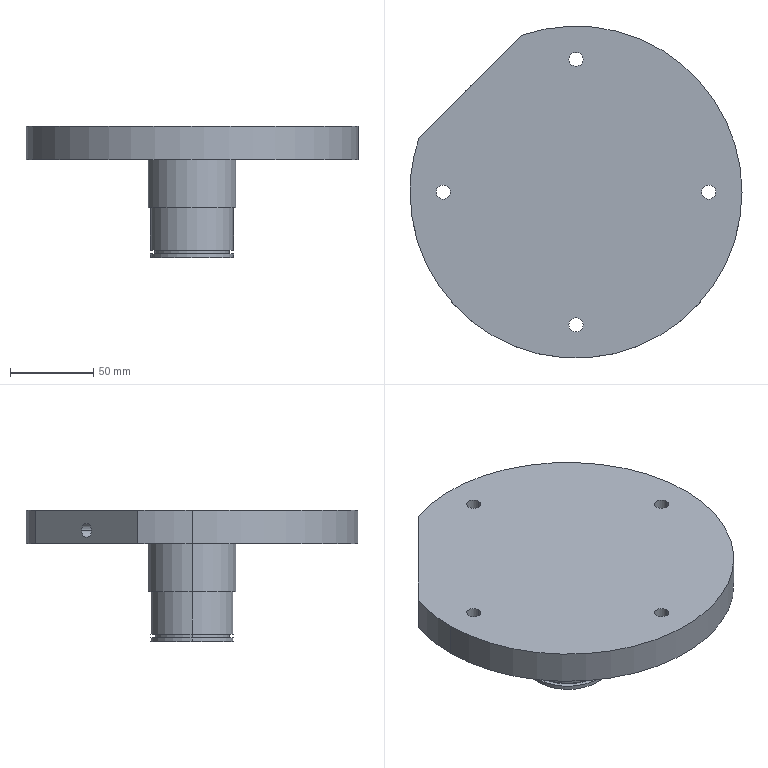Part | SolidWorks | features HoleWzd 2, ICE 2, CirPattern 1, Revolution 1 | 1 solid | 30 faces | box 200 x 200 x 79.02 mm | volume 730688 mm3 | cylinder 21 | plane 7 | cone 2 | commonest cylinder face diameters 8.5 x10 50 x4 200 x3 45 x2 53 x2
STEP:
#1=CARTESIAN_POINT('',(-18.208,24.218,-12.));
#2=VERTEX_POINT('',#1);
#3=CARTESIAN_POINT('',(-24.218,18.208,-12.));
#4=VERTEX_POINT('',#3);
#5=CARTESIAN_POINT('',(-21.213,21.213,-12.));
#6=DIRECTION('',(-0.7071,0.7071,0.));
#7=DIRECTION('',(-0.7071,-0.7071,0.));
#8=AXIS2_PLACEMENT_3D('',#5,#6,#7);
#9=CIRCLE('',#8,4.25);
#10=EDGE_CURVE('',#2,#4,#9,.T.);
#11=ORIENTED_EDGE('',*,*,#10,.F.);
#12=CARTESIAN_POINT('',(-60.634,66.645,-12.));
#13=VERTEX_POINT('',#12);
#14=CARTESIAN_POINT('',(-60.634,66.645,-12.));
#15=DIRECTION('',(-0.7071,0.7071,0.));
#16=VECTOR('',#15,1000.);
#17=LINE('',#14,#16);
#18=EDGE_CURVE('',#2,#13,#17,.T.);
#19=ORIENTED_EDGE('',*,*,#18,.T.);
#20=CARTESIAN_POINT('',(-66.645,60.634,-12.));
#21=VERTEX_POINT('',#20);
#22=CARTESIAN_POINT('',(-63.64,63.64,-12.));
#23=DIRECTION('',(-0.7071,0.7071,0.));
#24=DIRECTION('',(-0.7071,-0.7071,0.));
#25=AXIS2_PLACEMENT_3D('',#22,#23,#24);
#26=CIRCLE('',#25,4.25);
#27=EDGE_CURVE('',#13,#21,#26,.T.);
#28=ORIENTED_EDGE('',*,*,#27,.T.);
#29=CARTESIAN_POINT('',(-66.645,60.634,-12.));
#30=DIRECTION('',(-0.7071,0.7071,0.));
#31=VECTOR('',#30,1000.);
#32=LINE('',#29,#31);
#33=EDGE_CURVE('',#4,#21,#32,.T.);
#34=ORIENTED_EDGE('',*,*,#33,.F.);
#35=EDGE_LOOP('',(#11,#19,#28,#34));
#36=FACE_OUTER_BOUND('',#35,.T.);
#37=CARTESIAN_POINT('',(-63.64,63.64,-12.));
#38=DIRECTION('',(-0.7071,0.7071,0.));
#39=DIRECTION('',(-0.7071,-0.7071,0.));
#40=AXIS2_PLACEMENT_3D('',#37,#38,#39);
#41=CYLINDRICAL_SURFACE('',#40,4.25);
#42=ADVANCED_FACE('',(#36),#41,.F.);
#43=CARTESIAN_POINT('',(-19.407,19.407,-12.));
#44=VERTEX_POINT('',#43);
#45=CARTESIAN_POINT('',(-24.218,18.208,-12.));
#46=DIRECTION('',(-0.9703,-0.2419,0.));
#47=VECTOR('',#46,1000.);
#48=LINE('',#45,#47);
#49=EDGE_CURVE('',#44,#4,#48,.T.);
#50=ORIENTED_EDGE('',*,*,#49,.F.);
#51=CARTESIAN_POINT('',(-18.208,24.218,-12.));
#52=DIRECTION('',(0.2419,0.9703,0.));
#53=VECTOR('',#52,1000.);
#54=LINE('',#51,#53);
#55=EDGE_CURVE('',#44,#2,#54,.T.);
#56=ORIENTED_EDGE('',*,*,#55,.T.);
#57=ORIENTED_EDGE('',*,*,#10,.T.);
#58=EDGE_LOOP('',(#50,#56,#57));
#59=FACE_OUTER_BOUND('',#58,.T.);
#60=CARTESIAN_POINT('',(-21.213,21.213,-12.));
#61=DIRECTION('',(-0.7071,0.7071,0.));
#62=DIRECTION('',(-0.7071,-0.7071,0.));
#63=AXIS2_PLACEMENT_3D('',#60,#61,#62);
#64=CONICAL_SURFACE('',#63,4.25,1.03);
#65=ADVANCED_FACE('',(#59),#64,.F.);
#66=CARTESIAN_POINT('',(84.25,0.,0.));
#67=VERTEX_POINT('',#66);
#68=CARTESIAN_POINT('',(75.75,0.,0.));
#69=VERTEX_POINT('',#68);
#70=CARTESIAN_POINT('',(80.,0.,0.));
#71=DIRECTION('',(0.,0.,-1.));
#72=DIRECTION('',(-1.,0.,0.));
#73=AXIS2_PLACEMENT_3D('',#70,#71,#72);
#74=CIRCLE('',#73,4.25);
#75=EDGE_CURVE('',#67,#69,#74,.T.);
#76=ORIENTED_EDGE('',*,*,#75,.F.);
#77=CARTESIAN_POINT('',(84.25,0.,-20.));
#78=VERTEX_POINT('',#77);
#79=CARTESIAN_POINT('',(84.25,0.,-20.));
#80=DIRECTION('',(0.,0.,-1.));
#81=VECTOR('',#80,1000.);
#82=LINE('',#79,#81);
#83=EDGE_CURVE('',#67,#78,#82,.T.);
#84=ORIENTED_EDGE('',*,*,#83,.T.);
#85=CARTESIAN_POINT('',(75.75,0.,-20.));
#86=VERTEX_POINT('',#85);
#87=CARTESIAN_POINT('',(80.,0.,-20.));
#88=DIRECTION('',(0.,0.,-1.));
#89=DIRECTION('',(-1.,0.,0.));
#90=AXIS2_PLACEMENT_3D('',#87,#88,#89);
#91=CIRCLE('',#90,4.25);
#92=EDGE_CURVE('',#78,#86,#91,.T.);
#93=ORIENTED_EDGE('',*,*,#92,.T.);
#94=CARTESIAN_POINT('',(75.75,0.,-20.));
#95=DIRECTION('',(0.,0.,-1.));
#96=VECTOR('',#95,1000.);
#97=LINE('',#94,#96);
#98=EDGE_CURVE('',#69,#86,#97,.T.);
#99=ORIENTED_EDGE('',*,*,#98,.F.);
#100=EDGE_LOOP('',(#76,#84,#93,#99));
#101=FACE_OUTER_BOUND('',#100,.T.);
#102=CARTESIAN_POINT('',(80.,0.,-20.));
#103=DIRECTION('',(0.,0.,-1.));
#104=DIRECTION('',(-1.,0.,0.));
#105=AXIS2_PLACEMENT_3D('',#102,#103,#104);
#106=CYLINDRICAL_SURFACE('',#105,4.25);
#107=ADVANCED_FACE('',(#101),#106,.F.);
#108=CARTESIAN_POINT('',(4.25,80.,0.));
#109=VERTEX_POINT('',#108);
#110=CARTESIAN_POINT('',(-4.25,80.,0.));
#111=VERTEX_POINT('',#110);
#112=CARTESIAN_POINT('',(0.,80.,0.));
#113=DIRECTION('',(0.,0.,-1.));
#114=DIRECTION('',(-1.,0.,0.));
#115=AXIS2_PLACEMENT_3D('',#112,#113,#114);
#116=CIRCLE('',#115,4.25);
#117=EDGE_CURVE('',#109,#111,#116,.T.);
#118=ORIENTED_EDGE('',*,*,#117,.F.);
#119=CARTESIAN_POINT('',(4.25,80.,-20.));
#120=VERTEX_POINT('',#119);
#121=CARTESIAN_POINT('',(4.25,80.,-20.));
#122=DIRECTION('',(0.,0.,-1.));
#123=VECTOR('',#122,1000.);
#124=LINE('',#121,#123);
#125=EDGE_CURVE('',#109,#120,#124,.T.);
#126=ORIENTED_EDGE('',*,*,#125,.T.);
#127=CARTESIAN_POINT('',(-4.25,80.,-20.));
#128=VERTEX_POINT('',#127);
#129=CARTESIAN_POINT('',(0.,80.,-20.));
#130=DIRECTION('',(0.,0.,-1.));
#131=DIRECTION('',(-1.,0.,0.));
#132=AXIS2_PLACEMENT_3D('',#129,#130,#131);
#133=CIRCLE('',#132,4.25);
#134=EDGE_CURVE('',#120,#128,#133,.T.);
#135=ORIENTED_EDGE('',*,*,#134,.T.);
#136=CARTESIAN_POINT('',(-4.25,80.,-20.));
#137=DIRECTION('',(0.,0.,-1.));
#138=VECTOR('',#137,1000.);
#139=LINE('',#136,#138);
#140=EDGE_CURVE('',#111,#128,#139,.T.);
#141=ORIENTED_EDGE('',*,*,#140,.F.);
#142=EDGE_LOOP('',(#118,#126,#135,#141));
#143=FACE_OUTER_BOUND('',#142,.T.);
#144=CARTESIAN_POINT('',(0.,80.,-20.));
#145=DIRECTION('',(0.,0.,-1.));
#146=DIRECTION('',(-1.,0.,0.));
#147=AXIS2_PLACEMENT_3D('',#144,#145,#146);
#148=CYLINDRICAL_SURFACE('',#147,4.25);
#149=ADVANCED_FACE('',(#143),#148,.F.);
#150=CARTESIAN_POINT('',(-75.75,0.,0.));
#151=VERTEX_POINT('',#150);
#152=CARTESIAN_POINT('',(-84.25,0.,0.));
#153=VERTEX_POINT('',#152);
#154=CARTESIAN_POINT('',(-80.,0.,0.));
#155=DIRECTION('',(0.,0.,-1.));
#156=DIRECTION('',(-1.,0.,0.));
#157=AXIS2_PLACEMENT_3D('',#154,#155,#156);
#158=CIRCLE('',#157,4.25);
#159=EDGE_CURVE('',#151,#153,#158,.T.);
#160=ORIENTED_EDGE('',*,*,#159,.F.);
#161=CARTESIAN_POINT('',(-75.75,0.,-20.));
#162=VERTEX_POINT('',#161);
#163=CARTESIAN_POINT('',(-75.75,0.,-20.));
#164=DIRECTION('',(0.,0.,-1.));
#165=VECTOR('',#164,1000.);
#166=LINE('',#163,#165);
#167=EDGE_CURVE('',#151,#162,#166,.T.);
#168=ORIENTED_EDGE('',*,*,#167,.T.);
#169=CARTESIAN_POINT('',(-84.25,0.,-20.));
#170=VERTEX_POINT('',#169);
#171=CARTESIAN_POINT('',(-80.,0.,-20.));
#172=DIRECTION('',(0.,0.,-1.));
#173=DIRECTION('',(-1.,0.,0.));
#174=AXIS2_PLACEMENT_3D('',#171,#172,#173);
#175=CIRCLE('',#174,4.25);
#176=EDGE_CURVE('',#162,#170,#175,.T.);
#177=ORIENTED_EDGE('',*,*,#176,.T.);
#178=CARTESIAN_POINT('',(-84.25,0.,-20.));
#179=DIRECTION('',(0.,0.,-1.));
#180=VECTOR('',#179,1000.);
#181=LINE('',#178,#180);
#182=EDGE_CURVE('',#153,#170,#181,.T.);
#183=ORIENTED_EDGE('',*,*,#182,.F.);
#184=EDGE_LOOP('',(#160,#168,#177,#183));
#185=FACE_OUTER_BOUND('',#184,.T.);
#186=CARTESIAN_POINT('',(-80.,0.,-20.));
#187=DIRECTION('',(0.,0.,-1.));
#188=DIRECTION('',(-1.,0.,0.));
#189=AXIS2_PLACEMENT_3D('',#186,#187,#188);
#190=CYLINDRICAL_SURFACE('',#189,4.25);
#191=ADVANCED_FACE('',(#185),#190,.F.);
#192=CARTESIAN_POINT('',(4.25,-80.,0.));
#193=VERTEX_POINT('',#192);
#194=CARTESIAN_POINT('',(-4.25,-80.,0.));
#195=VERTEX_POINT('',#194);
#196=CARTESIAN_POINT('',(0.,-80.,0.));
#197=DIRECTION('',(0.,0.,-1.));
#198=DIRECTION('',(-1.,0.,0.));
#199=AXIS2_PLACEMENT_3D('',#196,#197,#198);
#200=CIRCLE('',#199,4.25);
#201=EDGE_CURVE('',#193,#195,#200,.T.);
#202=ORIENTED_EDGE('',*,*,#201,.F.);
#203=CARTESIAN_POINT('',(4.25,-80.,-20.));
#204=VERTEX_POINT('',#203);
#205=CARTESIAN_POINT('',(4.25,-80.,-20.));
#206=DIRECTION('',(0.,0.,-1.));
#207=VECTOR('',#206,1000.);
#208=LINE('',#205,#207);
#209=EDGE_CURVE('',#193,#204,#208,.T.);
#210=ORIENTED_EDGE('',*,*,#209,.T.);
#211=CARTESIAN_POINT('',(-4.25,-80.,-20.));
#212=VERTEX_POINT('',#211);
#213=CARTESIAN_POINT('',(0.,-80.,-20.));
#214=DIRECTION('',(0.,0.,-1.));
#215=DIRECTION('',(-1.,0.,0.));
#216=AXIS2_PLACEMENT_3D('',#213,#214,#215);
#217=CIRCLE('',#216,4.25);
#218=EDGE_CURVE('',#204,#212,#217,.T.);
#219=ORIENTED_EDGE('',*,*,#218,.T.);
#220=CARTESIAN_POINT('',(-4.25,-80.,-20.));
#221=DIRECTION('',(0.,0.,-1.));
#222=VECTOR('',#221,1000.);
#223=LINE('',#220,#222);
#224=EDGE_CURVE('',#195,#212,#223,.T.);
#225=ORIENTED_EDGE('',*,*,#224,.F.);
#226=EDGE_LOOP('',(#202,#210,#219,#225));
#227=FACE_OUTER_BOUND('',#226,.T.);
#228=CARTESIAN_POINT('',(0.,-80.,-20.));
#229=DIRECTION('',(0.,0.,-1.));
#230=DIRECTION('',(-1.,0.,0.));
#231=AXIS2_PLACEMENT_3D('',#228,#229,#230);
#232=CYLINDRICAL_SURFACE('',#231,4.25);
#233=ADVANCED_FACE('',(#227),#232,.F.);
#234=CARTESIAN_POINT('',(25.,0.,-76.72));
#235=VERTEX_POINT('',#234);
#236=CARTESIAN_POINT('',(-25.,0.,-76.72));
#237=VERTEX_POINT('',#236);
#238=CARTESIAN_POINT('',(0.,0.,-76.72));
#239=DIRECTION('',(0.,0.,1.));
#240=DIRECTION('',(-1.,0.,0.));
#241=AXIS2_PLACEMENT_3D('',#238,#239,#240);
#242=CIRCLE('',#241,25.);
#243=EDGE_CURVE('',#235,#237,#242,.T.);
#244=ORIENTED_EDGE('',*,*,#243,.F.);
#245=CARTESIAN_POINT('',(25.,0.,-79.02));
#246=VERTEX_POINT('',#245);
#247=CARTESIAN_POINT('',(25.,0.,0.));
#248=DIRECTION('',(0.,0.,-1.));
#249=VECTOR('',#248,1000.);
#250=LINE('',#247,#249);
#251=EDGE_CURVE('',#235,#246,#250,.T.);
#252=ORIENTED_EDGE('',*,*,#251,.T.);
#253=CARTESIAN_POINT('',(-25.,0.,-79.02));
#254=VERTEX_POINT('',#253);
#255=CARTESIAN_POINT('',(0.,0.,-79.02));
#256=DIRECTION('',(0.,0.,-1.));
#257=DIRECTION('',(-1.,0.,0.));
#258=AXIS2_PLACEMENT_3D('',#255,#256,#257);
#259=CIRCLE('',#258,25.);
#260=EDGE_CURVE('',#254,#246,#259,.T.);
#261=ORIENTED_EDGE('',*,*,#260,.F.);
#262=CARTESIAN_POINT('',(-25.,0.,0.));
#263=DIRECTION('',(0.,0.,-1.));
#264=VECTOR('',#263,1000.);
#265=LINE('',#262,#264);
#266=EDGE_CURVE('',#237,#254,#265,.T.);
#267=ORIENTED_EDGE('',*,*,#266,.F.);
#268=EDGE_LOOP('',(#244,#252,#261,#267));
#269=FACE_OUTER_BOUND('',#268,.T.);
#270=CARTESIAN_POINT('',(0.,0.,0.));
#271=DIRECTION('',(0.,0.,-1.));
#272=DIRECTION('',(-1.,0.,0.));
#273=AXIS2_PLACEMENT_3D('',#270,#271,#272);
#274=CYLINDRICAL_SURFACE('',#273,25.);
#275=ADVANCED_FACE('',(#269),#274,.T.);
#276=CARTESIAN_POINT('',(-22.5,0.,-76.72));
#277=VERTEX_POINT('',#276);
#278=CARTESIAN_POINT('',(22.5,0.,-76.72));
#279=VERTEX_POINT('',#278);
#280=CARTESIAN_POINT('',(0.,0.,-76.72));
#281=DIRECTION('',(0.,0.,-1.));
#282=DIRECTION('',(-1.,0.,0.));
#283=AXIS2_PLACEMENT_3D('',#280,#281,#282);
#284=CIRCLE('',#283,22.5);
#285=EDGE_CURVE('',#277,#279,#284,.T.);
#286=ORIENTED_EDGE('',*,*,#285,.F.);
#287=CARTESIAN_POINT('',(-22.5,0.,-74.52));
#288=VERTEX_POINT('',#287);
#289=CARTESIAN_POINT('',(-22.5,0.,-76.72));
#290=DIRECTION('',(0.,0.,1.));
#291=VECTOR('',#290,1000.);
#292=LINE('',#289,#291);
#293=EDGE_CURVE('',#277,#288,#292,.T.);
#294=ORIENTED_EDGE('',*,*,#293,.T.);
#295=CARTESIAN_POINT('',(22.5,0.,-74.52));
#296=VERTEX_POINT('',#295);
#297=CARTESIAN_POINT('',(0.,0.,-74.52));
#298=DIRECTION('',(0.,0.,-1.));
#299=DIRECTION('',(-1.,0.,0.));
#300=AXIS2_PLACEMENT_3D('',#297,#298,#299);
#301=CIRCLE('',#300,22.5);
#302=EDGE_CURVE('',#288,#296,#301,.T.);
#303=ORIENTED_EDGE('',*,*,#302,.T.);
#304=CARTESIAN_POINT('',(22.5,0.,-76.72));
#305=DIRECTION('',(0.,0.,1.));
#306=VECTOR('',#305,1000.);
#307=LINE('',#304,#306);
#308=EDGE_CURVE('',#279,#296,#307,.T.);
#309=ORIENTED_EDGE('',*,*,#308,.F.);
#310=EDGE_LOOP('',(#286,#294,#303,#309));
#311=FACE_OUTER_BOUND('',#310,.T.);
#312=CARTESIAN_POINT('',(0.,0.,-76.72));
#313=DIRECTION('',(0.,0.,1.));
#314=DIRECTION('',(1.,0.,0.));
#315=AXIS2_PLACEMENT_3D('',#312,#313,#314);
#316=CYLINDRICAL_SURFACE('',#315,22.5);
#317=ADVANCED_FACE('',(#311),#316,.T.);
#318=CARTESIAN_POINT('',(-26.5,0.,-20.));
#319=VERTEX_POINT('',#318);
#320=CARTESIAN_POINT('',(26.5,0.,-20.));
#321=VERTEX_POINT('',#320);
#322=CARTESIAN_POINT('',(0.,0.,-20.));
#323=DIRECTION('',(0.,0.,-1.));
#324=DIRECTION('',(-1.,0.,0.));
#325=AXIS2_PLACEMENT_3D('',#322,#323,#324);
#326=CIRCLE('',#325,26.5);
#327=EDGE_CURVE('',#319,#321,#326,.T.);
#328=ORIENTED_EDGE('',*,*,#327,.T.);
#329=CARTESIAN_POINT('',(26.5,0.,-49.02));
#330=VERTEX_POINT('',#329);
#331=CARTESIAN_POINT('',(26.5,0.,0.));
#332=DIRECTION('',(0.,0.,-1.));
#333=VECTOR('',#332,1000.);
#334=LINE('',#331,#333);
#335=EDGE_CURVE('',#321,#330,#334,.T.);
#336=ORIENTED_EDGE('',*,*,#335,.T.);
#337=CARTESIAN_POINT('',(-26.5,0.,-49.02));
#338=VERTEX_POINT('',#337);
#339=CARTESIAN_POINT('',(0.,0.,-49.02));
#340=DIRECTION('',(0.,0.,-1.));
#341=DIRECTION('',(-1.,0.,0.));
#342=AXIS2_PLACEMENT_3D('',#339,#340,#341);
#343=CIRCLE('',#342,26.5);
#344=EDGE_CURVE('',#338,#330,#343,.T.);
#345=ORIENTED_EDGE('',*,*,#344,.F.);
#346=CARTESIAN_POINT('',(-26.5,0.,0.));
#347=DIRECTION('',(0.,0.,-1.));
#348=VECTOR('',#347,1000.);
#349=LINE('',#346,#348);
#350=EDGE_CURVE('',#319,#338,#349,.T.);
#351=ORIENTED_EDGE('',*,*,#350,.F.);
#352=EDGE_LOOP('',(#328,#336,#345,#351));
#353=FACE_OUTER_BOUND('',#352,.T.);
#354=CARTESIAN_POINT('',(0.,0.,0.));
#355=DIRECTION('',(0.,0.,-1.));
#356=DIRECTION('',(-1.,0.,0.));
#357=AXIS2_PLACEMENT_3D('',#354,#355,#356);
#358=CYLINDRICAL_SURFACE('',#357,26.5);
#359=ADVANCED_FACE('',(#353),#358,.T.);
#360=CARTESIAN_POINT('',(-32.818,94.462,0.));
#361=VERTEX_POINT('',#360);
#362=CARTESIAN_POINT('',(100.,0.,0.));
#363=VERTEX_POINT('',#362);
#364=CARTESIAN_POINT('',(0.,0.,0.));
#365=DIRECTION('',(0.,0.,-1.));
#366=DIRECTION('',(-1.,0.,0.));
#367=AXIS2_PLACEMENT_3D('',#364,#365,#366);
#368=CIRCLE('',#367,100.);
#369=EDGE_CURVE('',#361,#363,#368,.T.);
#370=ORIENTED_EDGE('',*,*,#369,.T.);
#371=CARTESIAN_POINT('',(100.,0.,-20.));
#372=VERTEX_POINT('',#371);
#373=CARTESIAN_POINT('',(100.,0.,0.));
#374=DIRECTION('',(0.,0.,-1.));
#375=VECTOR('',#374,1000.);
#376=LINE('',#373,#375);
#377=EDGE_CURVE('',#363,#372,#376,.T.);
#378=ORIENTED_EDGE('',*,*,#377,.T.);
#379=CARTESIAN_POINT('',(-32.818,94.462,-20.));
#380=VERTEX_POINT('',#379);
#381=CARTESIAN_POINT('',(0.,0.,-20.));
#382=DIRECTION('',(0.,0.,-1.));
#383=DIRECTION('',(-1.,0.,0.));
#384=AXIS2_PLACEMENT_3D('',#381,#382,#383);
#385=CIRCLE('',#384,100.);
#386=EDGE_CURVE('',#380,#372,#385,.T.);
#387=ORIENTED_EDGE('',*,*,#386,.F.);
#388=CARTESIAN_POINT('',(-32.818,94.462,0.));
#389=DIRECTION('',(0.,0.,-1.));
#390=VECTOR('',#389,1000.);
#391=LINE('',#388,#390);
#392=EDGE_CURVE('',#361,#380,#391,.T.);
#393=ORIENTED_EDGE('',*,*,#392,.F.);
#394=EDGE_LOOP('',(#370,#378,#387,#393));
#395=FACE_OUTER_BOUND('',#394,.T.);
#396=CARTESIAN_POINT('',(0.,0.,0.));
#397=DIRECTION('',(0.,0.,-1.));
#398=DIRECTION('',(-1.,0.,0.));
#399=AXIS2_PLACEMENT_3D('',#396,#397,#398);
#400=CYLINDRICAL_SURFACE('',#399,100.);
#401=ADVANCED_FACE('',(#395),#400,.T.);
#402=ORIENTED_EDGE('',*,*,#377,.F.);
#403=CARTESIAN_POINT('',(-100.,0.,0.));
#404=VERTEX_POINT('',#403);
#405=CARTESIAN_POINT('',(0.,0.,0.));
#406=DIRECTION('',(0.,0.,-1.));
#407=DIRECTION('',(-1.,0.,0.));
#408=AXIS2_PLACEMENT_3D('',#405,#406,#407);
#409=CIRCLE('',#408,100.);
#410=EDGE_CURVE('',#363,#404,#409,.T.);
#411=ORIENTED_EDGE('',*,*,#410,.T.);
#412=CARTESIAN_POINT('',(-100.,0.,-20.));
#413=VERTEX_POINT('',#412);
#414=CARTESIAN_POINT('',(-100.,0.,0.));
#415=DIRECTION('',(0.,0.,-1.));
#416=VECTOR('',#415,1000.);
#417=LINE('',#414,#416);
#418=EDGE_CURVE('',#404,#413,#417,.T.);
#419=ORIENTED_EDGE('',*,*,#418,.T.);
#420=CARTESIAN_POINT('',(0.,0.,-20.));
#421=DIRECTION('',(0.,0.,-1.));
#422=DIRECTION('',(-1.,0.,0.));
#423=AXIS2_PLACEMENT_3D('',#420,#421,#422);
#424=CIRCLE('',#423,100.);
#425=EDGE_CURVE('',#372,#413,#424,.T.);
#426=ORIENTED_EDGE('',*,*,#425,.F.);
#427=EDGE_LOOP('',(#402,#411,#419,#426));
#428=FACE_OUTER_BOUND('',#427,.T.);
#429=CARTESIAN_POINT('',(0.,0.,0.));
#430=DIRECTION('',(0.,0.,-1.));
#431=DIRECTION('',(-1.,0.,0.));
#432=AXIS2_PLACEMENT_3D('',#429,#430,#431);
#433=CYLINDRICAL_SURFACE('',#432,100.);
#434=ADVANCED_FACE('',(#428),#433,.T.);
#435=CARTESIAN_POINT('',(-25.,0.,-49.02));
#436=VERTEX_POINT('',#435);
#437=CARTESIAN_POINT('',(25.,0.,-49.02));
#438=VERTEX_POINT('',#437);
#439=CARTESIAN_POINT('',(0.,0.,-49.02));
#440=DIRECTION('',(0.,0.,-1.));
#441=DIRECTION('',(-1.,0.,0.));
#442=AXIS2_PLACEMENT_3D('',#439,#440,#441);
#443=CIRCLE('',#442,25.);
#444=EDGE_CURVE('',#436,#438,#443,.T.);
#445=ORIENTED_EDGE('',*,*,#444,.T.);
#446=CARTESIAN_POINT('',(25.,0.,-74.52));
#447=VERTEX_POINT('',#446);
#448=CARTESIAN_POINT('',(25.,0.,0.));
#449=DIRECTION('',(0.,0.,-1.));
#450=VECTOR('',#449,1000.);
#451=LINE('',#448,#450);
#452=EDGE_CURVE('',#438,#447,#451,.T.);
#453=ORIENTED_EDGE('',*,*,#452,.T.);
#454=CARTESIAN_POINT('',(-25.,0.,-74.52));
#455=VERTEX_POINT('',#454);
#456=CARTESIAN_POINT('',(0.,0.,-74.52));
#457=DIRECTION('',(0.,0.,1.));
#458=DIRECTION('',(-1.,0.,0.));
#459=AXIS2_PLACEMENT_3D('',#456,#457,#458);
#460=CIRCLE('',#459,25.);
#461=EDGE_CURVE('',#447,#455,#460,.T.);
#462=ORIENTED_EDGE('',*,*,#461,.T.);
#463=CARTESIAN_POINT('',(-25.,0.,0.));
#464=DIRECTION('',(0.,0.,-1.));
#465=VECTOR('',#464,1000.);
#466=LINE('',#463,#465);
#467=EDGE_CURVE('',#436,#455,#466,.T.);
#468=ORIENTED_EDGE('',*,*,#467,.F.);
#469=EDGE_LOOP('',(#445,#453,#462,#468));
#470=FACE_OUTER_BOUND('',#469,.T.);
#471=CARTESIAN_POINT('',(0.,0.,0.));
#472=DIRECTION('',(0.,0.,-1.));
#473=DIRECTION('',(-1.,0.,0.));
#474=AXIS2_PLACEMENT_3D('',#471,#472,#473);
#475=CYLINDRICAL_SURFACE('',#474,25.);
#476=ADVANCED_FACE('',(#470),#475,.T.);
#477=ORIENTED_EDGE('',*,*,#452,.F.);
#478=CARTESIAN_POINT('',(0.,0.,-49.02));
#479=DIRECTION('',(0.,0.,-1.));
#480=DIRECTION('',(-1.,0.,0.));
#481=AXIS2_PLACEMENT_3D('',#478,#479,#480);
#482=CIRCLE('',#481,25.);
#483=EDGE_CURVE('',#438,#436,#482,.T.);
#484=ORIENTED_EDGE('',*,*,#483,.T.);
#485=ORIENTED_EDGE('',*,*,#467,.T.);
#486=CARTESIAN_POINT('',(0.,0.,-74.52));
#487=DIRECTION('',(0.,0.,1.));
#488=DIRECTION('',(-1.,0.,0.));
#489=AXIS2_PLACEMENT_3D('',#486,#487,#488);
#490=CIRCLE('',#489,25.);
#491=EDGE_CURVE('',#455,#447,#490,.T.);
#492=ORIENTED_EDGE('',*,*,#491,.T.);
#493=EDGE_LOOP('',(#477,#484,#485,#492));
#494=FACE_OUTER_BOUND('',#493,.T.);
#495=CARTESIAN_POINT('',(0.,0.,0.));
#496=DIRECTION('',(0.,0.,-1.));
#497=DIRECTION('',(-1.,0.,0.));
#498=AXIS2_PLACEMENT_3D('',#495,#496,#497);
#499=CYLINDRICAL_SURFACE('',#498,25.);
#500=ADVANCED_FACE('',(#494),#499,.T.);
#501=CARTESIAN_POINT('',(-94.462,32.818,0.));
#502=VERTEX_POINT('',#501);
#503=CARTESIAN_POINT('',(-106.066,21.213,0.));
#504=DIRECTION('',(-0.7071,-0.7071,0.));
#505=VECTOR('',#504,1000.);
#506=LINE('',#503,#505);
#507=EDGE_CURVE('',#361,#502,#506,.T.);
#508=ORIENTED_EDGE('',*,*,#507,.T.);
#509=CARTESIAN_POINT('',(0.,0.,0.));
#510=DIRECTION('',(0.,0.,-1.));
#511=DIRECTION('',(-1.,0.,0.));
#512=AXIS2_PLACEMENT_3D('',#509,#510,#511);
#513=CIRCLE('',#512,100.);
#514=EDGE_CURVE('',#404,#502,#513,.T.);
#515=ORIENTED_EDGE('',*,*,#514,.F.);
#516=ORIENTED_EDGE('',*,*,#410,.F.);
#517=ORIENTED_EDGE('',*,*,#369,.F.);
#518=EDGE_LOOP('',(#508,#515,#516,#517));
#519=FACE_OUTER_BOUND('',#518,.T.);
#520=CARTESIAN_POINT('',(80.,0.,0.));
#521=DIRECTION('',(0.,0.,-1.));
#522=DIRECTION('',(-1.,0.,0.));
#523=AXIS2_PLACEMENT_3D('',#520,#521,#522);
#524=CIRCLE('',#523,4.25);
#525=EDGE_CURVE('',#69,#67,#524,.T.);
#526=ORIENTED_EDGE('',*,*,#525,.T.);
#527=ORIENTED_EDGE('',*,*,#75,.T.);
#528=EDGE_LOOP('',(#526,#527));
#529=FACE_BOUND('',#528,.T.);
#530=CARTESIAN_POINT('',(0.,80.,0.));
#531=DIRECTION('',(0.,0.,-1.));
#532=DIRECTION('',(-1.,0.,0.));
#533=AXIS2_PLACEMENT_3D('',#530,#531,#532);
#534=CIRCLE('',#533,4.25);
#535=EDGE_CURVE('',#111,#109,#534,.T.);
#536=ORIENTED_EDGE('',*,*,#535,.T.);
#537=ORIENTED_EDGE('',*,*,#117,.T.);
#538=EDGE_LOOP('',(#536,#537));
#539=FACE_BOUND('',#538,.T.);
#540=CARTESIAN_POINT('',(-80.,0.,0.));
#541=DIRECTION('',(0.,0.,-1.));
#542=DIRECTION('',(-1.,0.,0.));
#543=AXIS2_PLACEMENT_3D('',#540,#541,#542);
#544=CIRCLE('',#543,4.25);
#545=EDGE_CURVE('',#153,#151,#544,.T.);
#546=ORIENTED_EDGE('',*,*,#545,.T.);
#547=ORIENTED_EDGE('',*,*,#159,.T.);
#548=EDGE_LOOP('',(#546,#547));
#549=FACE_BOUND('',#548,.T.);
#550=CARTESIAN_POINT('',(0.,-80.,0.));
#551=DIRECTION('',(0.,0.,-1.));
#552=DIRECTION('',(-1.,0.,0.));
#553=AXIS2_PLACEMENT_3D('',#550,#551,#552);
#554=CIRCLE('',#553,4.25);
#555=EDGE_CURVE('',#195,#193,#554,.T.);
#556=ORIENTED_EDGE('',*,*,#555,.T.);
#557=ORIENTED_EDGE('',*,*,#201,.T.);
#558=EDGE_LOOP('',(#556,#557));
#559=FACE_BOUND('',#558,.T.);
#560=CARTESIAN_POINT('',(0.,0.,0.));
#561=DIRECTION('',(0.,0.,1.));
#562=DIRECTION('',(1.,0.,0.));
#563=AXIS2_PLACEMENT_3D('',#560,#561,#562);
#564=PLANE('',#563);
#565=ADVANCED_FACE('',(#519,#529,#539,#549,#559),#564,.T.);
#566=ORIENTED_EDGE('',*,*,#418,.F.);
#567=ORIENTED_EDGE('',*,*,#514,.T.);
#568=CARTESIAN_POINT('',(-94.462,32.818,-20.));
#569=VERTEX_POINT('',#568);
#570=CARTESIAN_POINT('',(-94.462,32.818,0.));
#571=DIRECTION('',(0.,0.,1.));
#572=VECTOR('',#571,1000.);
#573=LINE('',#570,#572);
#574=EDGE_CURVE('',#569,#502,#573,.T.);
#575=ORIENTED_EDGE('',*,*,#574,.F.);
#576=CARTESIAN_POINT('',(0.,0.,-20.));
#577=DIRECTION('',(0.,0.,-1.));
#578=DIRECTION('',(-1.,0.,0.));
#579=AXIS2_PLACEMENT_3D('',#576,#577,#578);
#580=CIRCLE('',#579,100.);
#581=EDGE_CURVE('',#413,#569,#580,.T.);
#582=ORIENTED_EDGE('',*,*,#581,.F.);
#583=EDGE_LOOP('',(#566,#567,#575,#582));
#584=FACE_OUTER_BOUND('',#583,.T.);
#585=CARTESIAN_POINT('',(0.,0.,0.));
#586=DIRECTION('',(0.,0.,-1.));
#587=DIRECTION('',(-1.,0.,0.));
#588=AXIS2_PLACEMENT_3D('',#585,#586,#587);
#589=CYLINDRICAL_SURFACE('',#588,100.);
#590=ADVANCED_FACE('',(#584),#589,.T.);
#591=CARTESIAN_POINT('',(-113.64,13.64,-20.));
#592=DIRECTION('',(-0.7071,-0.7071,0.));
#593=VECTOR('',#592,1000.);
#594=LINE('',#591,#593);
#595=EDGE_CURVE('',#380,#569,#594,.T.);
#596=ORIENTED_EDGE('',*,*,#595,.F.);
#597=ORIENTED_EDGE('',*,*,#386,.T.);
#598=ORIENTED_EDGE('',*,*,#425,.T.);
#599=ORIENTED_EDGE('',*,*,#581,.T.);
#600=EDGE_LOOP('',(#596,#597,#598,#599));
#601=FACE_OUTER_BOUND('',#600,.T.);
#602=CARTESIAN_POINT('',(80.,0.,-20.));
#603=DIRECTION('',(0.,0.,-1.));
#604=DIRECTION('',(-1.,0.,0.));
#605=AXIS2_PLACEMENT_3D('',#602,#603,#604);
#606=CIRCLE('',#605,4.25);
#607=EDGE_CURVE('',#86,#78,#606,.T.);
#608=ORIENTED_EDGE('',*,*,#607,.F.);
#609=ORIENTED_EDGE('',*,*,#92,.F.);
#610=EDGE_LOOP('',(#608,#609));
#611=FACE_BOUND('',#610,.T.);
#612=CARTESIAN_POINT('',(0.,80.,-20.));
#613=DIRECTION('',(0.,0.,-1.));
#614=DIRECTION('',(-1.,0.,0.));
#615=AXIS2_PLACEMENT_3D('',#612,#613,#614);
#616=CIRCLE('',#615,4.25);
#617=EDGE_CURVE('',#128,#120,#616,.T.);
#618=ORIENTED_EDGE('',*,*,#617,.F.);
#619=ORIENTED_EDGE('',*,*,#134,.F.);
#620=EDGE_LOOP('',(#618,#619));
#621=FACE_BOUND('',#620,.T.);
#622=CARTESIAN_POINT('',(-80.,0.,-20.));
#623=DIRECTION('',(0.,0.,-1.));
#624=DIRECTION('',(-1.,0.,0.));
#625=AXIS2_PLACEMENT_3D('',#622,#623,#624);
#626=CIRCLE('',#625,4.25);
#627=EDGE_CURVE('',#170,#162,#626,.T.);
#628=ORIENTED_EDGE('',*,*,#627,.F.);
#629=ORIENTED_EDGE('',*,*,#176,.F.);
#630=EDGE_LOOP('',(#628,#629));
#631=FACE_BOUND('',#630,.T.);
#632=CARTESIAN_POINT('',(0.,-80.,-20.));
#633=DIRECTION('',(0.,0.,-1.));
#634=DIRECTION('',(-1.,0.,0.));
#635=AXIS2_PLACEMENT_3D('',#632,#633,#634);
#636=CIRCLE('',#635,4.25);
#637=EDGE_CURVE('',#212,#204,#636,.T.);
#638=ORIENTED_EDGE('',*,*,#637,.F.);
#639=ORIENTED_EDGE('',*,*,#218,.F.);
#640=EDGE_LOOP('',(#638,#639));
#641=FACE_BOUND('',#640,.T.);
#642=ORIENTED_EDGE('',*,*,#327,.F.);
#643=CARTESIAN_POINT('',(0.,0.,-20.));
#644=DIRECTION('',(0.,0.,-1.));
#645=DIRECTION('',(-1.,0.,0.));
#646=AXIS2_PLACEMENT_3D('',#643,#644,#645);
#647=CIRCLE('',#646,26.5);
#648=EDGE_CURVE('',#321,#319,#647,.T.);
#649=ORIENTED_EDGE('',*,*,#648,.F.);
#650=EDGE_LOOP('',(#642,#649));
#651=FACE_BOUND('',#650,.T.);
#652=CARTESIAN_POINT('',(-100.,0.,-20.));
#653=DIRECTION('',(0.,0.,-1.));
#654=DIRECTION('',(-1.,0.,0.));
#655=AXIS2_PLACEMENT_3D('',#652,#653,#654);
#656=PLANE('',#655);
#657=ADVANCED_FACE('',(#601,#611,#621,#631,#641,#651),#656,.T.);
#658=ORIENTED_EDGE('',*,*,#335,.F.);
#659=ORIENTED_EDGE('',*,*,#648,.T.);
#660=ORIENTED_EDGE('',*,*,#350,.T.);
#661=CARTESIAN_POINT('',(0.,0.,-49.02));
#662=DIRECTION('',(0.,0.,-1.));
#663=DIRECTION('',(-1.,0.,0.));
#664=AXIS2_PLACEMENT_3D('',#661,#662,#663);
#665=CIRCLE('',#664,26.5);
#666=EDGE_CURVE('',#330,#338,#665,.T.);
#667=ORIENTED_EDGE('',*,*,#666,.F.);
#668=EDGE_LOOP('',(#658,#659,#660,#667));
#669=FACE_OUTER_BOUND('',#668,.T.);
#670=CARTESIAN_POINT('',(0.,0.,0.));
#671=DIRECTION('',(0.,0.,-1.));
#672=DIRECTION('',(-1.,0.,0.));
#673=AXIS2_PLACEMENT_3D('',#670,#671,#672);
#674=CYLINDRICAL_SURFACE('',#673,26.5);
#675=ADVANCED_FACE('',(#669),#674,.T.);
#676=ORIENTED_EDGE('',*,*,#344,.T.);
#677=ORIENTED_EDGE('',*,*,#666,.T.);
#678=EDGE_LOOP('',(#676,#677));
#679=FACE_OUTER_BOUND('',#678,.T.);
#680=ORIENTED_EDGE('',*,*,#444,.F.);
#681=ORIENTED_EDGE('',*,*,#483,.F.);
#682=EDGE_LOOP('',(#680,#681));
#683=FACE_BOUND('',#682,.T.);
#684=CARTESIAN_POINT('',(-26.5,0.,-49.02));
#685=DIRECTION('',(0.,0.,-1.));
#686=DIRECTION('',(-1.,0.,0.));
#687=AXIS2_PLACEMENT_3D('',#684,#685,#686);
#688=PLANE('',#687);
#689=ADVANCED_FACE('',(#679,#683),#688,.T.);
#690=CARTESIAN_POINT('',(0.,0.,-76.72));
#691=DIRECTION('',(0.,0.,1.));
#692=DIRECTION('',(-1.,0.,0.));
#693=AXIS2_PLACEMENT_3D('',#690,#691,#692);
#694=CIRCLE('',#693,25.);
#695=EDGE_CURVE('',#237,#235,#694,.T.);
#696=ORIENTED_EDGE('',*,*,#695,.T.);
#697=ORIENTED_EDGE('',*,*,#243,.T.);
#698=EDGE_LOOP('',(#696,#697));
#699=FACE_OUTER_BOUND('',#698,.T.);
#700=CARTESIAN_POINT('',(0.,0.,-76.72));
#701=DIRECTION('',(0.,0.,-1.));
#702=DIRECTION('',(-1.,0.,0.));
#703=AXIS2_PLACEMENT_3D('',#700,#701,#702);
#704=CIRCLE('',#703,22.5);
#705=EDGE_CURVE('',#279,#277,#704,.T.);
#706=ORIENTED_EDGE('',*,*,#705,.T.);
#707=ORIENTED_EDGE('',*,*,#285,.T.);
#708=EDGE_LOOP('',(#706,#707));
#709=FACE_BOUND('',#708,.T.);
#710=CARTESIAN_POINT('',(0.,0.,-76.72));
#711=DIRECTION('',(0.,0.,-1.));
#712=DIRECTION('',(-1.,0.,0.));
#713=AXIS2_PLACEMENT_3D('',#710,#711,#712);
#714=PLANE('',#713);
#715=ADVANCED_FACE('',(#699,#709),#714,.F.);
#716=ORIENTED_EDGE('',*,*,#491,.F.);
#717=ORIENTED_EDGE('',*,*,#461,.F.);
#718=EDGE_LOOP('',(#716,#717));
#719=FACE_OUTER_BOUND('',#718,.T.);
#720=CARTESIAN_POINT('',(0.,0.,-74.52));
#721=DIRECTION('',(0.,0.,-1.));
#722=DIRECTION('',(-1.,0.,0.));
#723=AXIS2_PLACEMENT_3D('',#720,#721,#722);
#724=CIRCLE('',#723,22.5);
#725=EDGE_CURVE('',#296,#288,#724,.T.);
#726=ORIENTED_EDGE('',*,*,#725,.F.);
#727=ORIENTED_EDGE('',*,*,#302,.F.);
#728=EDGE_LOOP('',(#726,#727));
#729=FACE_BOUND('',#728,.T.);
#730=CARTESIAN_POINT('',(0.,0.,-74.52));
#731=DIRECTION('',(0.,0.,-1.));
#732=DIRECTION('',(-1.,0.,0.));
#733=AXIS2_PLACEMENT_3D('',#730,#731,#732);
#734=PLANE('',#733);
#735=ADVANCED_FACE('',(#719,#729),#734,.T.);
#736=ORIENTED_EDGE('',*,*,#293,.F.);
#737=ORIENTED_EDGE('',*,*,#705,.F.);
#738=ORIENTED_EDGE('',*,*,#308,.T.);
#739=ORIENTED_EDGE('',*,*,#725,.T.);
#740=EDGE_LOOP('',(#736,#737,#738,#739));
#741=FACE_OUTER_BOUND('',#740,.T.);
#742=CARTESIAN_POINT('',(0.,0.,-76.72));
#743=DIRECTION('',(0.,0.,1.));
#744=DIRECTION('',(1.,0.,0.));
#745=AXIS2_PLACEMENT_3D('',#742,#743,#744);
#746=CYLINDRICAL_SURFACE('',#745,22.5);
#747=ADVANCED_FACE('',(#741),#746,.T.);
#748=ORIENTED_EDGE('',*,*,#260,.T.);
#749=CARTESIAN_POINT('',(0.,0.,-79.02));
#750=DIRECTION('',(0.,0.,-1.));
#751=DIRECTION('',(-1.,0.,0.));
#752=AXIS2_PLACEMENT_3D('',#749,#750,#751);
#753=CIRCLE('',#752,25.);
#754=EDGE_CURVE('',#246,#254,#753,.T.);
#755=ORIENTED_EDGE('',*,*,#754,.T.);
#756=EDGE_LOOP('',(#748,#755));
#757=FACE_OUTER_BOUND('',#756,.T.);
#758=CARTESIAN_POINT('',(-25.,0.,-79.02));
#759=DIRECTION('',(0.,0.,-1.));
#760=DIRECTION('',(-1.,0.,0.));
#761=AXIS2_PLACEMENT_3D('',#758,#759,#760);
#762=PLANE('',#761);
#763=ADVANCED_FACE('',(#757),#762,.T.);
#764=ORIENTED_EDGE('',*,*,#251,.F.);
#765=ORIENTED_EDGE('',*,*,#695,.F.);
#766=ORIENTED_EDGE('',*,*,#266,.T.);
#767=ORIENTED_EDGE('',*,*,#754,.F.);
#768=EDGE_LOOP('',(#764,#765,#766,#767));
#769=FACE_OUTER_BOUND('',#768,.T.);
#770=CARTESIAN_POINT('',(0.,0.,0.));
#771=DIRECTION('',(0.,0.,-1.));
#772=DIRECTION('',(-1.,0.,0.));
#773=AXIS2_PLACEMENT_3D('',#770,#771,#772);
#774=CYLINDRICAL_SURFACE('',#773,25.);
#775=ADVANCED_FACE('',(#769),#774,.T.);
#776=ORIENTED_EDGE('',*,*,#209,.F.);
#777=ORIENTED_EDGE('',*,*,#555,.F.);
#778=ORIENTED_EDGE('',*,*,#224,.T.);
#779=ORIENTED_EDGE('',*,*,#637,.T.);
#780=EDGE_LOOP('',(#776,#777,#778,#779));
#781=FACE_OUTER_BOUND('',#780,.T.);
#782=CARTESIAN_POINT('',(0.,-80.,-20.));
#783=DIRECTION('',(0.,0.,-1.));
#784=DIRECTION('',(-1.,0.,0.));
#785=AXIS2_PLACEMENT_3D('',#782,#783,#784);
#786=CYLINDRICAL_SURFACE('',#785,4.25);
#787=ADVANCED_FACE('',(#781),#786,.F.);
#788=ORIENTED_EDGE('',*,*,#167,.F.);
#789=ORIENTED_EDGE('',*,*,#545,.F.);
#790=ORIENTED_EDGE('',*,*,#182,.T.);
#791=ORIENTED_EDGE('',*,*,#627,.T.);
#792=EDGE_LOOP('',(#788,#789,#790,#791));
#793=FACE_OUTER_BOUND('',#792,.T.);
#794=CARTESIAN_POINT('',(-80.,0.,-20.));
#795=DIRECTION('',(0.,0.,-1.));
#796=DIRECTION('',(-1.,0.,0.));
#797=AXIS2_PLACEMENT_3D('',#794,#795,#796);
#798=CYLINDRICAL_SURFACE('',#797,4.25);
#799=ADVANCED_FACE('',(#793),#798,.F.);
#800=ORIENTED_EDGE('',*,*,#125,.F.);
#801=ORIENTED_EDGE('',*,*,#535,.F.);
#802=ORIENTED_EDGE('',*,*,#140,.T.);
#803=ORIENTED_EDGE('',*,*,#617,.T.);
#804=EDGE_LOOP('',(#800,#801,#802,#803));
#805=FACE_OUTER_BOUND('',#804,.T.);
#806=CARTESIAN_POINT('',(0.,80.,-20.));
#807=DIRECTION('',(0.,0.,-1.));
#808=DIRECTION('',(-1.,0.,0.));
#809=AXIS2_PLACEMENT_3D('',#806,#807,#808);
#810=CYLINDRICAL_SURFACE('',#809,4.25);
#811=ADVANCED_FACE('',(#805),#810,.F.);
#812=ORIENTED_EDGE('',*,*,#83,.F.);
#813=ORIENTED_EDGE('',*,*,#525,.F.);
#814=ORIENTED_EDGE('',*,*,#98,.T.);
#815=ORIENTED_EDGE('',*,*,#607,.T.);
#816=EDGE_LOOP('',(#812,#813,#814,#815));
#817=FACE_OUTER_BOUND('',#816,.T.);
#818=CARTESIAN_POINT('',(80.,0.,-20.));
#819=DIRECTION('',(0.,0.,-1.));
#820=DIRECTION('',(-1.,0.,0.));
#821=AXIS2_PLACEMENT_3D('',#818,#819,#820);
#822=CYLINDRICAL_SURFACE('',#821,4.25);
#823=ADVANCED_FACE('',(#817),#822,.F.);
#824=CARTESIAN_POINT('',(-63.64,63.64,-12.));
#825=DIRECTION('',(-0.7071,0.7071,0.));
#826=DIRECTION('',(-0.7071,-0.7071,0.));
#827=AXIS2_PLACEMENT_3D('',#824,#825,#826);
#828=CIRCLE('',#827,4.25);
#829=EDGE_CURVE('',#21,#13,#828,.T.);
#830=ORIENTED_EDGE('',*,*,#829,.F.);
#831=ORIENTED_EDGE('',*,*,#27,.F.);
#832=EDGE_LOOP('',(#830,#831));
#833=FACE_BOUND('',#832,.T.);
#834=ORIENTED_EDGE('',*,*,#574,.T.);
#835=ORIENTED_EDGE('',*,*,#507,.F.);
#836=ORIENTED_EDGE('',*,*,#392,.T.);
#837=ORIENTED_EDGE('',*,*,#595,.T.);
#838=EDGE_LOOP('',(#834,#835,#836,#837));
#839=FACE_OUTER_BOUND('',#838,.T.);
#840=CARTESIAN_POINT('',(-106.066,21.213,0.));
#841=DIRECTION('',(0.7071,-0.7071,0.));
#842=DIRECTION('',(0.7071,0.7071,0.));
#843=AXIS2_PLACEMENT_3D('',#840,#841,#842);
#844=PLANE('',#843);
#845=ADVANCED_FACE('',(#833,#839),#844,.F.);
#846=ORIENTED_EDGE('',*,*,#55,.F.);
#847=ORIENTED_EDGE('',*,*,#49,.T.);
#848=CARTESIAN_POINT('',(-21.213,21.213,-12.));
#849=DIRECTION('',(-0.7071,0.7071,0.));
#850=DIRECTION('',(-0.7071,-0.7071,0.));
#851=AXIS2_PLACEMENT_3D('',#848,#849,#850);
#852=CIRCLE('',#851,4.25);
#853=EDGE_CURVE('',#4,#2,#852,.T.);
#854=ORIENTED_EDGE('',*,*,#853,.T.);
#855=EDGE_LOOP('',(#846,#847,#854));
#856=FACE_OUTER_BOUND('',#855,.T.);
#857=CARTESIAN_POINT('',(-21.213,21.213,-12.));
#858=DIRECTION('',(-0.7071,0.7071,0.));
#859=DIRECTION('',(-0.7071,-0.7071,0.));
#860=AXIS2_PLACEMENT_3D('',#857,#858,#859);
#861=CONICAL_SURFACE('',#860,4.25,1.03);
#862=ADVANCED_FACE('',(#856),#861,.F.);
#863=ORIENTED_EDGE('',*,*,#18,.F.);
#864=ORIENTED_EDGE('',*,*,#853,.F.);
#865=ORIENTED_EDGE('',*,*,#33,.T.);
#866=ORIENTED_EDGE('',*,*,#829,.T.);
#867=EDGE_LOOP('',(#863,#864,#865,#866));
#868=FACE_OUTER_BOUND('',#867,.T.);
#869=CARTESIAN_POINT('',(-63.64,63.64,-12.));
#870=DIRECTION('',(-0.7071,0.7071,0.));
#871=DIRECTION('',(-0.7071,-0.7071,0.));
#872=AXIS2_PLACEMENT_3D('',#869,#870,#871);
#873=CYLINDRICAL_SURFACE('',#872,4.25);
#874=ADVANCED_FACE('',(#868),#873,.F.);
#875=CLOSED_SHELL('',(#42,#65,#107,#149,#191,#233,#275,#317,#359,#401,#434,#476,#500,#565,#590,#657,#675,#689,#715,#735,#747,#763,#775,#787,#799,#811,#823,#845,#862,#874));
#876=MANIFOLD_SOLID_BREP('',#875);
#877=CARTESIAN_POINT('',(0.,0.,0.));
#878=DIRECTION('',(0.,0.,1.));
#879=DIRECTION('',(1.,0.,0.));
#880=AXIS2_PLACEMENT_3D('',#877,#878,#879);
#881=(LENGTH_UNIT()NAMED_UNIT(*)SI_UNIT(.MILLI.,.METRE.));
#882=UNCERTAINTY_MEASURE_WITH_UNIT(LENGTH_MEASURE(0.00001),#881,'','');
#883=(NAMED_UNIT(*)PLANE_ANGLE_UNIT()SI_UNIT($,.RADIAN.));
#884=(NAMED_UNIT(*)SI_UNIT($,.STERADIAN.)SOLID_ANGLE_UNIT());
#885=(GEOMETRIC_REPRESENTATION_CONTEXT(3)GLOBAL_UNCERTAINTY_ASSIGNED_CONTEXT((#882))GLOBAL_UNIT_ASSIGNED_CONTEXT((#881,#883,#884))REPRESENTATION_CONTEXT('',''));
#886=ADVANCED_BREP_SHAPE_REPRESENTATION('',(#876,#880),#885);